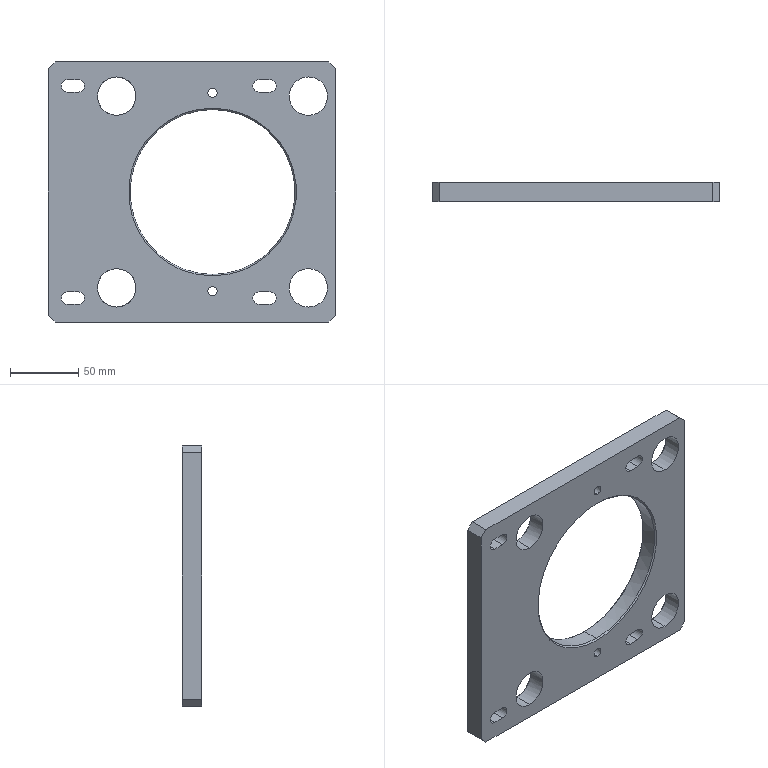Part | STEP file | PN_0015 Pre-compression sleeve guide seat | 1 solid | 116 faces | box 210 x 14 x 190 mm | volume 352968 mm3 | cylinder 54 | cone 44 | plane 18 | commonest cylinder face diameters 3.3 x32 9 x8 28 x8 6.8 x4 120.5 x2